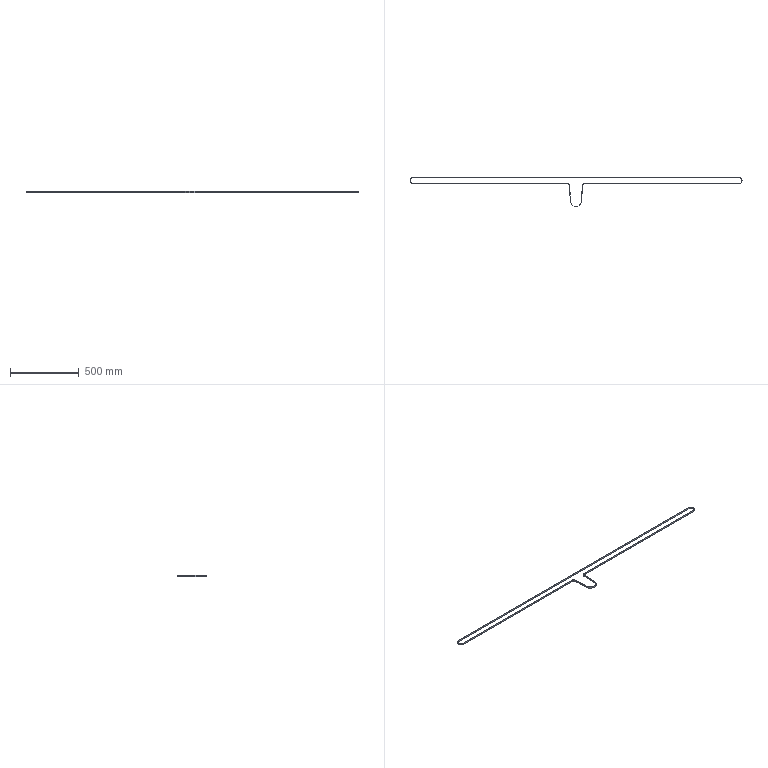Part | NX | features BREP 1 | 1 solid | 24 faces | box 2421 x 214.1 x 12 mm | volume 74422 mm3 | cylinder 12 | plane 12 | commonest cylinder face diameters 45 x3 47.4 x3 25 x2 27.4 x2 80 x1 82.4 x1
STEP:
#1=CARTESIAN_POINT('',(1728.714,8.857,-2.25));
#2=VERTEX_POINT('',#1);
#3=CARTESIAN_POINT('',(1706.214,31.357,-2.25));
#4=VERTEX_POINT('',#3);
#5=CARTESIAN_POINT('',(1706.214,8.857,-2.25));
#6=DIRECTION('',(0.,0.,1.));
#7=DIRECTION('',(-1.,0.,0.));
#8=AXIS2_PLACEMENT_3D('',#5,#6,#7);
#9=CIRCLE('',#8,22.5);
#10=EDGE_CURVE('',#2,#4,#9,.T.);
#11=ORIENTED_EDGE('',*,*,#10,.F.);
#12=CARTESIAN_POINT('',(1728.714,8.857,9.75));
#13=VERTEX_POINT('',#12);
#14=CARTESIAN_POINT('',(1728.714,8.857,-2.25));
#15=DIRECTION('',(0.,0.,1.));
#16=VECTOR('',#15,1000.);
#17=LINE('',#14,#16);
#18=EDGE_CURVE('',#2,#13,#17,.T.);
#19=ORIENTED_EDGE('',*,*,#18,.T.);
#20=CARTESIAN_POINT('',(1706.214,31.357,9.75));
#21=VERTEX_POINT('',#20);
#22=CARTESIAN_POINT('',(1706.214,8.857,9.75));
#23=DIRECTION('',(0.,0.,1.));
#24=DIRECTION('',(-1.,0.,0.));
#25=AXIS2_PLACEMENT_3D('',#22,#23,#24);
#26=CIRCLE('',#25,22.5);
#27=EDGE_CURVE('',#13,#21,#26,.T.);
#28=ORIENTED_EDGE('',*,*,#27,.T.);
#29=CARTESIAN_POINT('',(1706.214,31.357,-2.25));
#30=DIRECTION('',(0.,0.,1.));
#31=VECTOR('',#30,1000.);
#32=LINE('',#29,#31);
#33=EDGE_CURVE('',#4,#21,#32,.T.);
#34=ORIENTED_EDGE('',*,*,#33,.F.);
#35=EDGE_LOOP('',(#11,#19,#28,#34));
#36=FACE_BOUND('',#35,.T.);
#37=CARTESIAN_POINT('',(1706.214,8.857,-2.25));
#38=DIRECTION('',(0.,0.,1.));
#39=DIRECTION('',(1.,0.,0.));
#40=AXIS2_PLACEMENT_3D('',#37,#38,#39);
#41=CYLINDRICAL_SURFACE('',#40,22.5);
#42=ADVANCED_FACE('',(#36),#41,.F.);
#43=CARTESIAN_POINT('',(1706.214,-14.843,-2.25));
#44=VERTEX_POINT('',#43);
#45=CARTESIAN_POINT('',(1729.914,8.857,-2.25));
#46=VERTEX_POINT('',#45);
#47=CARTESIAN_POINT('',(1706.214,8.857,-2.25));
#48=DIRECTION('',(0.,0.,1.));
#49=DIRECTION('',(1.,0.,0.));
#50=AXIS2_PLACEMENT_3D('',#47,#48,#49);
#51=CIRCLE('',#50,23.7);
#52=EDGE_CURVE('',#44,#46,#51,.T.);
#53=ORIENTED_EDGE('',*,*,#52,.T.);
#54=CARTESIAN_POINT('',(1729.914,8.857,9.75));
#55=VERTEX_POINT('',#54);
#56=CARTESIAN_POINT('',(1729.914,8.857,-2.25));
#57=DIRECTION('',(0.,0.,1.));
#58=VECTOR('',#57,1000.);
#59=LINE('',#56,#58);
#60=EDGE_CURVE('',#46,#55,#59,.T.);
#61=ORIENTED_EDGE('',*,*,#60,.T.);
#62=CARTESIAN_POINT('',(1706.214,-14.843,9.75));
#63=VERTEX_POINT('',#62);
#64=CARTESIAN_POINT('',(1706.214,8.857,9.75));
#65=DIRECTION('',(0.,0.,1.));
#66=DIRECTION('',(1.,0.,0.));
#67=AXIS2_PLACEMENT_3D('',#64,#65,#66);
#68=CIRCLE('',#67,23.7);
#69=EDGE_CURVE('',#63,#55,#68,.T.);
#70=ORIENTED_EDGE('',*,*,#69,.F.);
#71=CARTESIAN_POINT('',(1706.214,-14.843,-2.25));
#72=DIRECTION('',(0.,0.,1.));
#73=VECTOR('',#72,1000.);
#74=LINE('',#71,#73);
#75=EDGE_CURVE('',#44,#63,#74,.T.);
#76=ORIENTED_EDGE('',*,*,#75,.F.);
#77=EDGE_LOOP('',(#53,#61,#70,#76));
#78=FACE_BOUND('',#77,.T.);
#79=CARTESIAN_POINT('',(1706.214,8.857,-2.25));
#80=DIRECTION('',(0.,0.,1.));
#81=DIRECTION('',(1.,0.,0.));
#82=AXIS2_PLACEMENT_3D('',#79,#80,#81);
#83=CYLINDRICAL_SURFACE('',#82,23.7);
#84=ADVANCED_FACE('',(#78),#83,.T.);
#85=ORIENTED_EDGE('',*,*,#60,.F.);
#86=CARTESIAN_POINT('',(1706.214,32.557,-2.25));
#87=VERTEX_POINT('',#86);
#88=CARTESIAN_POINT('',(1706.214,8.857,-2.25));
#89=DIRECTION('',(0.,0.,1.));
#90=DIRECTION('',(1.,0.,0.));
#91=AXIS2_PLACEMENT_3D('',#88,#89,#90);
#92=CIRCLE('',#91,23.7);
#93=EDGE_CURVE('',#46,#87,#92,.T.);
#94=ORIENTED_EDGE('',*,*,#93,.T.);
#95=CARTESIAN_POINT('',(1706.214,32.557,9.75));
#96=VERTEX_POINT('',#95);
#97=CARTESIAN_POINT('',(1706.214,32.557,-2.25));
#98=DIRECTION('',(0.,0.,1.));
#99=VECTOR('',#98,1000.);
#100=LINE('',#97,#99);
#101=EDGE_CURVE('',#87,#96,#100,.T.);
#102=ORIENTED_EDGE('',*,*,#101,.T.);
#103=CARTESIAN_POINT('',(1706.214,8.857,9.75));
#104=DIRECTION('',(0.,0.,1.));
#105=DIRECTION('',(1.,0.,0.));
#106=AXIS2_PLACEMENT_3D('',#103,#104,#105);
#107=CIRCLE('',#106,23.7);
#108=EDGE_CURVE('',#55,#96,#107,.T.);
#109=ORIENTED_EDGE('',*,*,#108,.F.);
#110=EDGE_LOOP('',(#85,#94,#102,#109));
#111=FACE_BOUND('',#110,.T.);
#112=CARTESIAN_POINT('',(1706.214,8.857,-2.25));
#113=DIRECTION('',(0.,0.,1.));
#114=DIRECTION('',(1.,0.,0.));
#115=AXIS2_PLACEMENT_3D('',#112,#113,#114);
#116=CYLINDRICAL_SURFACE('',#115,23.7);
#117=ADVANCED_FACE('',(#111),#116,.T.);
#118=CARTESIAN_POINT('',(579.214,-14.843,9.75));
#119=VERTEX_POINT('',#118);
#120=CARTESIAN_POINT('',(579.214,-14.843,9.75));
#121=DIRECTION('',(1.,0.,0.));
#122=VECTOR('',#121,1000.);
#123=LINE('',#120,#122);
#124=EDGE_CURVE('',#119,#63,#123,.T.);
#125=ORIENTED_EDGE('',*,*,#124,.F.);
#126=CARTESIAN_POINT('',(579.214,-14.843,-2.25));
#127=VERTEX_POINT('',#126);
#128=CARTESIAN_POINT('',(579.214,-14.843,-2.25));
#129=DIRECTION('',(0.,0.,1.));
#130=VECTOR('',#129,1000.);
#131=LINE('',#128,#130);
#132=EDGE_CURVE('',#127,#119,#131,.T.);
#133=ORIENTED_EDGE('',*,*,#132,.F.);
#134=CARTESIAN_POINT('',(579.214,-14.843,-2.25));
#135=DIRECTION('',(1.,0.,0.));
#136=VECTOR('',#135,1000.);
#137=LINE('',#134,#136);
#138=EDGE_CURVE('',#127,#44,#137,.T.);
#139=ORIENTED_EDGE('',*,*,#138,.T.);
#140=ORIENTED_EDGE('',*,*,#75,.T.);
#141=EDGE_LOOP('',(#125,#133,#139,#140));
#142=FACE_BOUND('',#141,.T.);
#143=CARTESIAN_POINT('',(579.214,-14.843,-2.25));
#144=DIRECTION('',(0.,-1.,0.));
#145=DIRECTION('',(0.,0.,-1.));
#146=AXIS2_PLACEMENT_3D('',#143,#144,#145);
#147=PLANE('',#146);
#148=ADVANCED_FACE('',(#142),#147,.T.);
#149=CARTESIAN_POINT('',(566.733,-26.656,9.75));
#150=VERTEX_POINT('',#149);
#151=CARTESIAN_POINT('',(579.214,-27.343,9.75));
#152=DIRECTION('',(0.,0.,-1.));
#153=DIRECTION('',(-1.,0.,0.));
#154=AXIS2_PLACEMENT_3D('',#151,#152,#153);
#155=CIRCLE('',#154,12.5);
#156=EDGE_CURVE('',#150,#119,#155,.T.);
#157=ORIENTED_EDGE('',*,*,#156,.F.);
#158=CARTESIAN_POINT('',(566.733,-26.656,-2.25));
#159=VERTEX_POINT('',#158);
#160=CARTESIAN_POINT('',(566.733,-26.656,-2.25));
#161=DIRECTION('',(0.,0.,1.));
#162=VECTOR('',#161,1000.);
#163=LINE('',#160,#162);
#164=EDGE_CURVE('',#159,#150,#163,.T.);
#165=ORIENTED_EDGE('',*,*,#164,.F.);
#166=CARTESIAN_POINT('',(579.214,-27.343,-2.25));
#167=DIRECTION('',(0.,0.,-1.));
#168=DIRECTION('',(-1.,0.,0.));
#169=AXIS2_PLACEMENT_3D('',#166,#167,#168);
#170=CIRCLE('',#169,12.5);
#171=EDGE_CURVE('',#159,#127,#170,.T.);
#172=ORIENTED_EDGE('',*,*,#171,.T.);
#173=ORIENTED_EDGE('',*,*,#132,.T.);
#174=EDGE_LOOP('',(#157,#165,#172,#173));
#175=FACE_BOUND('',#174,.T.);
#176=CARTESIAN_POINT('',(579.214,-27.343,-2.25));
#177=DIRECTION('',(0.,0.,1.));
#178=DIRECTION('',(1.,0.,0.));
#179=AXIS2_PLACEMENT_3D('',#176,#177,#178);
#180=CYLINDRICAL_SURFACE('',#179,12.5);
#181=ADVANCED_FACE('',(#175),#180,.F.);
#182=CARTESIAN_POINT('',(560.352,-142.607,9.75));
#183=VERTEX_POINT('',#182);
#184=CARTESIAN_POINT('',(560.352,-142.607,9.75));
#185=DIRECTION('',(0.05495,0.9985,0.));
#186=VECTOR('',#185,1000.);
#187=LINE('',#184,#186);
#188=EDGE_CURVE('',#183,#150,#187,.T.);
#189=ORIENTED_EDGE('',*,*,#188,.F.);
#190=CARTESIAN_POINT('',(560.352,-142.607,-2.25));
#191=VERTEX_POINT('',#190);
#192=CARTESIAN_POINT('',(560.352,-142.607,-2.25));
#193=DIRECTION('',(0.,0.,1.));
#194=VECTOR('',#193,1000.);
#195=LINE('',#192,#194);
#196=EDGE_CURVE('',#191,#183,#195,.T.);
#197=ORIENTED_EDGE('',*,*,#196,.F.);
#198=CARTESIAN_POINT('',(560.352,-142.607,-2.25));
#199=DIRECTION('',(0.05495,0.9985,0.));
#200=VECTOR('',#199,1000.);
#201=LINE('',#198,#200);
#202=EDGE_CURVE('',#191,#159,#201,.T.);
#203=ORIENTED_EDGE('',*,*,#202,.T.);
#204=ORIENTED_EDGE('',*,*,#164,.T.);
#205=EDGE_LOOP('',(#189,#197,#203,#204));
#206=FACE_BOUND('',#205,.T.);
#207=CARTESIAN_POINT('',(560.352,-142.607,-2.25));
#208=DIRECTION('',(0.9985,-0.05495,0.));
#209=DIRECTION('',(0.,0.,-1.));
#210=AXIS2_PLACEMENT_3D('',#207,#208,#209);
#211=PLANE('',#210);
#212=ADVANCED_FACE('',(#206),#211,.T.);
#213=CARTESIAN_POINT('',(478.077,-142.607,9.75));
#214=VERTEX_POINT('',#213);
#215=CARTESIAN_POINT('',(519.214,-140.343,9.75));
#216=DIRECTION('',(0.,0.,1.));
#217=DIRECTION('',(1.,0.,0.));
#218=AXIS2_PLACEMENT_3D('',#215,#216,#217);
#219=CIRCLE('',#218,41.2);
#220=EDGE_CURVE('',#214,#183,#219,.T.);
#221=ORIENTED_EDGE('',*,*,#220,.F.);
#222=CARTESIAN_POINT('',(478.077,-142.607,-2.25));
#223=VERTEX_POINT('',#222);
#224=CARTESIAN_POINT('',(478.077,-142.607,-2.25));
#225=DIRECTION('',(0.,0.,1.));
#226=VECTOR('',#225,1000.);
#227=LINE('',#224,#226);
#228=EDGE_CURVE('',#223,#214,#227,.T.);
#229=ORIENTED_EDGE('',*,*,#228,.F.);
#230=CARTESIAN_POINT('',(519.214,-140.343,-2.25));
#231=DIRECTION('',(0.,0.,1.));
#232=DIRECTION('',(1.,0.,0.));
#233=AXIS2_PLACEMENT_3D('',#230,#231,#232);
#234=CIRCLE('',#233,41.2);
#235=EDGE_CURVE('',#223,#191,#234,.T.);
#236=ORIENTED_EDGE('',*,*,#235,.T.);
#237=ORIENTED_EDGE('',*,*,#196,.T.);
#238=EDGE_LOOP('',(#221,#229,#236,#237));
#239=FACE_BOUND('',#238,.T.);
#240=CARTESIAN_POINT('',(519.214,-140.343,-2.25));
#241=DIRECTION('',(0.,0.,1.));
#242=DIRECTION('',(1.,0.,0.));
#243=AXIS2_PLACEMENT_3D('',#240,#241,#242);
#244=CYLINDRICAL_SURFACE('',#243,41.2);
#245=ADVANCED_FACE('',(#239),#244,.T.);
#246=CARTESIAN_POINT('',(471.695,-26.656,9.75));
#247=VERTEX_POINT('',#246);
#248=CARTESIAN_POINT('',(471.695,-26.656,9.75));
#249=DIRECTION('',(0.05495,-0.9985,0.));
#250=VECTOR('',#249,1000.);
#251=LINE('',#248,#250);
#252=EDGE_CURVE('',#247,#214,#251,.T.);
#253=ORIENTED_EDGE('',*,*,#252,.F.);
#254=CARTESIAN_POINT('',(471.695,-26.656,-2.25));
#255=VERTEX_POINT('',#254);
#256=CARTESIAN_POINT('',(471.695,-26.656,-2.25));
#257=DIRECTION('',(0.,0.,1.));
#258=VECTOR('',#257,1000.);
#259=LINE('',#256,#258);
#260=EDGE_CURVE('',#255,#247,#259,.T.);
#261=ORIENTED_EDGE('',*,*,#260,.F.);
#262=CARTESIAN_POINT('',(471.695,-26.656,-2.25));
#263=DIRECTION('',(0.05495,-0.9985,0.));
#264=VECTOR('',#263,1000.);
#265=LINE('',#262,#264);
#266=EDGE_CURVE('',#255,#223,#265,.T.);
#267=ORIENTED_EDGE('',*,*,#266,.T.);
#268=ORIENTED_EDGE('',*,*,#228,.T.);
#269=EDGE_LOOP('',(#253,#261,#267,#268));
#270=FACE_BOUND('',#269,.T.);
#271=CARTESIAN_POINT('',(471.695,-26.656,-2.25));
#272=DIRECTION('',(-0.9985,-0.05495,0.));
#273=DIRECTION('',(-0.05495,0.9985,0.));
#274=AXIS2_PLACEMENT_3D('',#271,#272,#273);
#275=PLANE('',#274);
#276=ADVANCED_FACE('',(#270),#275,.T.);
#277=CARTESIAN_POINT('',(459.214,-14.843,9.75));
#278=VERTEX_POINT('',#277);
#279=CARTESIAN_POINT('',(459.214,-27.343,9.75));
#280=DIRECTION('',(0.,0.,-1.));
#281=DIRECTION('',(-1.,0.,0.));
#282=AXIS2_PLACEMENT_3D('',#279,#280,#281);
#283=CIRCLE('',#282,12.5);
#284=EDGE_CURVE('',#278,#247,#283,.T.);
#285=ORIENTED_EDGE('',*,*,#284,.F.);
#286=CARTESIAN_POINT('',(459.214,-14.843,-2.25));
#287=VERTEX_POINT('',#286);
#288=CARTESIAN_POINT('',(459.214,-14.843,-2.25));
#289=DIRECTION('',(0.,0.,1.));
#290=VECTOR('',#289,1000.);
#291=LINE('',#288,#290);
#292=EDGE_CURVE('',#287,#278,#291,.T.);
#293=ORIENTED_EDGE('',*,*,#292,.F.);
#294=CARTESIAN_POINT('',(459.214,-27.343,-2.25));
#295=DIRECTION('',(0.,0.,-1.));
#296=DIRECTION('',(-1.,0.,0.));
#297=AXIS2_PLACEMENT_3D('',#294,#295,#296);
#298=CIRCLE('',#297,12.5);
#299=EDGE_CURVE('',#287,#255,#298,.T.);
#300=ORIENTED_EDGE('',*,*,#299,.T.);
#301=ORIENTED_EDGE('',*,*,#260,.T.);
#302=EDGE_LOOP('',(#285,#293,#300,#301));
#303=FACE_BOUND('',#302,.T.);
#304=CARTESIAN_POINT('',(459.214,-27.343,-2.25));
#305=DIRECTION('',(0.,0.,1.));
#306=DIRECTION('',(1.,0.,0.));
#307=AXIS2_PLACEMENT_3D('',#304,#305,#306);
#308=CYLINDRICAL_SURFACE('',#307,12.5);
#309=ADVANCED_FACE('',(#303),#308,.F.);
#310=CARTESIAN_POINT('',(-667.786,-14.843,9.75));
#311=VERTEX_POINT('',#310);
#312=CARTESIAN_POINT('',(-667.786,-14.843,9.75));
#313=DIRECTION('',(1.,0.,0.));
#314=VECTOR('',#313,1000.);
#315=LINE('',#312,#314);
#316=EDGE_CURVE('',#311,#278,#315,.T.);
#317=ORIENTED_EDGE('',*,*,#316,.F.);
#318=CARTESIAN_POINT('',(-667.786,-14.843,-2.25));
#319=VERTEX_POINT('',#318);
#320=CARTESIAN_POINT('',(-667.786,-14.843,-2.25));
#321=DIRECTION('',(0.,0.,1.));
#322=VECTOR('',#321,1000.);
#323=LINE('',#320,#322);
#324=EDGE_CURVE('',#319,#311,#323,.T.);
#325=ORIENTED_EDGE('',*,*,#324,.F.);
#326=CARTESIAN_POINT('',(-667.786,-14.843,-2.25));
#327=DIRECTION('',(1.,0.,0.));
#328=VECTOR('',#327,1000.);
#329=LINE('',#326,#328);
#330=EDGE_CURVE('',#319,#287,#329,.T.);
#331=ORIENTED_EDGE('',*,*,#330,.T.);
#332=ORIENTED_EDGE('',*,*,#292,.T.);
#333=EDGE_LOOP('',(#317,#325,#331,#332));
#334=FACE_BOUND('',#333,.T.);
#335=CARTESIAN_POINT('',(-667.786,-14.843,-2.25));
#336=DIRECTION('',(0.,-1.,0.));
#337=DIRECTION('',(-1.,0.,0.));
#338=AXIS2_PLACEMENT_3D('',#335,#336,#337);
#339=PLANE('',#338);
#340=ADVANCED_FACE('',(#334),#339,.T.);
#341=CARTESIAN_POINT('',(-667.786,32.557,9.75));
#342=VERTEX_POINT('',#341);
#343=CARTESIAN_POINT('',(-667.786,8.857,9.75));
#344=DIRECTION('',(0.,0.,1.));
#345=DIRECTION('',(1.,0.,0.));
#346=AXIS2_PLACEMENT_3D('',#343,#344,#345);
#347=CIRCLE('',#346,23.7);
#348=EDGE_CURVE('',#342,#311,#347,.T.);
#349=ORIENTED_EDGE('',*,*,#348,.F.);
#350=CARTESIAN_POINT('',(-667.786,32.557,-2.25));
#351=VERTEX_POINT('',#350);
#352=CARTESIAN_POINT('',(-667.786,32.557,-2.25));
#353=DIRECTION('',(0.,0.,1.));
#354=VECTOR('',#353,1000.);
#355=LINE('',#352,#354);
#356=EDGE_CURVE('',#351,#342,#355,.T.);
#357=ORIENTED_EDGE('',*,*,#356,.F.);
#358=CARTESIAN_POINT('',(-667.786,8.857,-2.25));
#359=DIRECTION('',(0.,0.,1.));
#360=DIRECTION('',(1.,0.,0.));
#361=AXIS2_PLACEMENT_3D('',#358,#359,#360);
#362=CIRCLE('',#361,23.7);
#363=EDGE_CURVE('',#351,#319,#362,.T.);
#364=ORIENTED_EDGE('',*,*,#363,.T.);
#365=ORIENTED_EDGE('',*,*,#324,.T.);
#366=EDGE_LOOP('',(#349,#357,#364,#365));
#367=FACE_BOUND('',#366,.T.);
#368=CARTESIAN_POINT('',(-667.786,8.857,-2.25));
#369=DIRECTION('',(0.,0.,1.));
#370=DIRECTION('',(1.,0.,0.));
#371=AXIS2_PLACEMENT_3D('',#368,#369,#370);
#372=CYLINDRICAL_SURFACE('',#371,23.7);
#373=ADVANCED_FACE('',(#367),#372,.T.);
#374=CARTESIAN_POINT('',(1706.214,32.557,9.75));
#375=DIRECTION('',(-1.,0.,0.));
#376=VECTOR('',#375,1000.);
#377=LINE('',#374,#376);
#378=EDGE_CURVE('',#96,#342,#377,.T.);
#379=ORIENTED_EDGE('',*,*,#378,.F.);
#380=ORIENTED_EDGE('',*,*,#101,.F.);
#381=CARTESIAN_POINT('',(1706.214,32.557,-2.25));
#382=DIRECTION('',(-1.,0.,0.));
#383=VECTOR('',#382,1000.);
#384=LINE('',#381,#383);
#385=EDGE_CURVE('',#87,#351,#384,.T.);
#386=ORIENTED_EDGE('',*,*,#385,.T.);
#387=ORIENTED_EDGE('',*,*,#356,.T.);
#388=EDGE_LOOP('',(#379,#380,#386,#387));
#389=FACE_BOUND('',#388,.T.);
#390=CARTESIAN_POINT('',(1706.214,32.557,-2.25));
#391=DIRECTION('',(0.,1.,0.));
#392=DIRECTION('',(1.,0.,0.));
#393=AXIS2_PLACEMENT_3D('',#390,#391,#392);
#394=PLANE('',#393);
#395=ADVANCED_FACE('',(#389),#394,.T.);
#396=ORIENTED_EDGE('',*,*,#52,.F.);
#397=ORIENTED_EDGE('',*,*,#138,.F.);
#398=ORIENTED_EDGE('',*,*,#171,.F.);
#399=ORIENTED_EDGE('',*,*,#202,.F.);
#400=ORIENTED_EDGE('',*,*,#235,.F.);
#401=ORIENTED_EDGE('',*,*,#266,.F.);
#402=ORIENTED_EDGE('',*,*,#299,.F.);
#403=ORIENTED_EDGE('',*,*,#330,.F.);
#404=ORIENTED_EDGE('',*,*,#363,.F.);
#405=ORIENTED_EDGE('',*,*,#385,.F.);
#406=ORIENTED_EDGE('',*,*,#93,.F.);
#407=EDGE_LOOP('',(#396,#397,#398,#399,#400,#401,#402,#403,#404,#405,#406));
#408=FACE_BOUND('',#407,.T.);
#409=CARTESIAN_POINT('',(472.894,-26.59,-2.25));
#410=VERTEX_POINT('',#409);
#411=CARTESIAN_POINT('',(479.275,-142.541,-2.25));
#412=VERTEX_POINT('',#411);
#413=CARTESIAN_POINT('',(479.275,-142.541,-2.25));
#414=DIRECTION('',(0.05495,-0.9985,0.));
#415=VECTOR('',#414,1000.);
#416=LINE('',#413,#415);
#417=EDGE_CURVE('',#410,#412,#416,.T.);
#418=ORIENTED_EDGE('',*,*,#417,.T.);
#419=CARTESIAN_POINT('',(559.154,-142.541,-2.25));
#420=VERTEX_POINT('',#419);
#421=CARTESIAN_POINT('',(519.214,-140.343,-2.25));
#422=DIRECTION('',(0.,0.,1.));
#423=DIRECTION('',(-1.,0.,0.));
#424=AXIS2_PLACEMENT_3D('',#421,#422,#423);
#425=CIRCLE('',#424,40.);
#426=EDGE_CURVE('',#412,#420,#425,.T.);
#427=ORIENTED_EDGE('',*,*,#426,.T.);
#428=CARTESIAN_POINT('',(565.535,-26.59,-2.25));
#429=VERTEX_POINT('',#428);
#430=CARTESIAN_POINT('',(565.535,-26.59,-2.25));
#431=DIRECTION('',(0.05495,0.9985,0.));
#432=VECTOR('',#431,1000.);
#433=LINE('',#430,#432);
#434=EDGE_CURVE('',#420,#429,#433,.T.);
#435=ORIENTED_EDGE('',*,*,#434,.T.);
#436=CARTESIAN_POINT('',(579.214,-13.643,-2.25));
#437=VERTEX_POINT('',#436);
#438=CARTESIAN_POINT('',(579.214,-27.343,-2.25));
#439=DIRECTION('',(0.,0.,-1.));
#440=DIRECTION('',(1.,0.,0.));
#441=AXIS2_PLACEMENT_3D('',#438,#439,#440);
#442=CIRCLE('',#441,13.7);
#443=EDGE_CURVE('',#429,#437,#442,.T.);
#444=ORIENTED_EDGE('',*,*,#443,.T.);
#445=CARTESIAN_POINT('',(1706.214,-13.643,-2.25));
#446=VERTEX_POINT('',#445);
#447=CARTESIAN_POINT('',(1706.214,-13.643,-2.25));
#448=DIRECTION('',(1.,0.,0.));
#449=VECTOR('',#448,1000.);
#450=LINE('',#447,#449);
#451=EDGE_CURVE('',#437,#446,#450,.T.);
#452=ORIENTED_EDGE('',*,*,#451,.T.);
#453=CARTESIAN_POINT('',(1706.214,8.857,-2.25));
#454=DIRECTION('',(0.,0.,1.));
#455=DIRECTION('',(-1.,0.,0.));
#456=AXIS2_PLACEMENT_3D('',#453,#454,#455);
#457=CIRCLE('',#456,22.5);
#458=EDGE_CURVE('',#446,#2,#457,.T.);
#459=ORIENTED_EDGE('',*,*,#458,.T.);
#460=ORIENTED_EDGE('',*,*,#10,.T.);
#461=CARTESIAN_POINT('',(-667.786,31.357,-2.25));
#462=VERTEX_POINT('',#461);
#463=CARTESIAN_POINT('',(-667.786,31.357,-2.25));
#464=DIRECTION('',(-1.,0.,0.));
#465=VECTOR('',#464,1000.);
#466=LINE('',#463,#465);
#467=EDGE_CURVE('',#4,#462,#466,.T.);
#468=ORIENTED_EDGE('',*,*,#467,.T.);
#469=CARTESIAN_POINT('',(-667.786,-13.643,-2.25));
#470=VERTEX_POINT('',#469);
#471=CARTESIAN_POINT('',(-667.786,8.857,-2.25));
#472=DIRECTION('',(0.,0.,1.));
#473=DIRECTION('',(-1.,0.,0.));
#474=AXIS2_PLACEMENT_3D('',#471,#472,#473);
#475=CIRCLE('',#474,22.5);
#476=EDGE_CURVE('',#462,#470,#475,.T.);
#477=ORIENTED_EDGE('',*,*,#476,.T.);
#478=CARTESIAN_POINT('',(459.214,-13.643,-2.25));
#479=VERTEX_POINT('',#478);
#480=CARTESIAN_POINT('',(459.214,-13.643,-2.25));
#481=DIRECTION('',(1.,0.,0.));
#482=VECTOR('',#481,1000.);
#483=LINE('',#480,#482);
#484=EDGE_CURVE('',#470,#479,#483,.T.);
#485=ORIENTED_EDGE('',*,*,#484,.T.);
#486=CARTESIAN_POINT('',(459.214,-27.343,-2.25));
#487=DIRECTION('',(0.,0.,-1.));
#488=DIRECTION('',(1.,0.,0.));
#489=AXIS2_PLACEMENT_3D('',#486,#487,#488);
#490=CIRCLE('',#489,13.7);
#491=EDGE_CURVE('',#479,#410,#490,.T.);
#492=ORIENTED_EDGE('',*,*,#491,.T.);
#493=EDGE_LOOP('',(#418,#427,#435,#444,#452,#459,#460,#468,#477,#485,#492));
#494=FACE_BOUND('',#493,.T.);
#495=CARTESIAN_POINT('',(1706.214,8.857,-2.25));
#496=DIRECTION('',(0.,0.,1.));
#497=DIRECTION('',(1.,0.,0.));
#498=AXIS2_PLACEMENT_3D('',#495,#496,#497);
#499=PLANE('',#498);
#500=ADVANCED_FACE('',(#408,#494),#499,.F.);
#501=ORIENTED_EDGE('',*,*,#69,.T.);
#502=ORIENTED_EDGE('',*,*,#108,.T.);
#503=ORIENTED_EDGE('',*,*,#378,.T.);
#504=ORIENTED_EDGE('',*,*,#348,.T.);
#505=ORIENTED_EDGE('',*,*,#316,.T.);
#506=ORIENTED_EDGE('',*,*,#284,.T.);
#507=ORIENTED_EDGE('',*,*,#252,.T.);
#508=ORIENTED_EDGE('',*,*,#220,.T.);
#509=ORIENTED_EDGE('',*,*,#188,.T.);
#510=ORIENTED_EDGE('',*,*,#156,.T.);
#511=ORIENTED_EDGE('',*,*,#124,.T.);
#512=EDGE_LOOP('',(#501,#502,#503,#504,#505,#506,#507,#508,#509,#510,#511));
#513=FACE_BOUND('',#512,.T.);
#514=CARTESIAN_POINT('',(479.275,-142.541,9.75));
#515=VERTEX_POINT('',#514);
#516=CARTESIAN_POINT('',(559.154,-142.541,9.75));
#517=VERTEX_POINT('',#516);
#518=CARTESIAN_POINT('',(519.214,-140.343,9.75));
#519=DIRECTION('',(0.,0.,1.));
#520=DIRECTION('',(-1.,0.,0.));
#521=AXIS2_PLACEMENT_3D('',#518,#519,#520);
#522=CIRCLE('',#521,40.);
#523=EDGE_CURVE('',#515,#517,#522,.T.);
#524=ORIENTED_EDGE('',*,*,#523,.F.);
#525=CARTESIAN_POINT('',(472.894,-26.59,9.75));
#526=VERTEX_POINT('',#525);
#527=CARTESIAN_POINT('',(479.275,-142.541,9.75));
#528=DIRECTION('',(0.05495,-0.9985,0.));
#529=VECTOR('',#528,1000.);
#530=LINE('',#527,#529);
#531=EDGE_CURVE('',#526,#515,#530,.T.);
#532=ORIENTED_EDGE('',*,*,#531,.F.);
#533=CARTESIAN_POINT('',(459.214,-13.643,9.75));
#534=VERTEX_POINT('',#533);
#535=CARTESIAN_POINT('',(459.214,-27.343,9.75));
#536=DIRECTION('',(0.,0.,-1.));
#537=DIRECTION('',(1.,0.,0.));
#538=AXIS2_PLACEMENT_3D('',#535,#536,#537);
#539=CIRCLE('',#538,13.7);
#540=EDGE_CURVE('',#534,#526,#539,.T.);
#541=ORIENTED_EDGE('',*,*,#540,.F.);
#542=CARTESIAN_POINT('',(-667.786,-13.643,9.75));
#543=VERTEX_POINT('',#542);
#544=CARTESIAN_POINT('',(459.214,-13.643,9.75));
#545=DIRECTION('',(1.,0.,0.));
#546=VECTOR('',#545,1000.);
#547=LINE('',#544,#546);
#548=EDGE_CURVE('',#543,#534,#547,.T.);
#549=ORIENTED_EDGE('',*,*,#548,.F.);
#550=CARTESIAN_POINT('',(-667.786,31.357,9.75));
#551=VERTEX_POINT('',#550);
#552=CARTESIAN_POINT('',(-667.786,8.857,9.75));
#553=DIRECTION('',(0.,0.,1.));
#554=DIRECTION('',(-1.,0.,0.));
#555=AXIS2_PLACEMENT_3D('',#552,#553,#554);
#556=CIRCLE('',#555,22.5);
#557=EDGE_CURVE('',#551,#543,#556,.T.);
#558=ORIENTED_EDGE('',*,*,#557,.F.);
#559=CARTESIAN_POINT('',(-667.786,31.357,9.75));
#560=DIRECTION('',(-1.,0.,0.));
#561=VECTOR('',#560,1000.);
#562=LINE('',#559,#561);
#563=EDGE_CURVE('',#21,#551,#562,.T.);
#564=ORIENTED_EDGE('',*,*,#563,.F.);
#565=ORIENTED_EDGE('',*,*,#27,.F.);
#566=CARTESIAN_POINT('',(1706.214,-13.643,9.75));
#567=VERTEX_POINT('',#566);
#568=CARTESIAN_POINT('',(1706.214,8.857,9.75));
#569=DIRECTION('',(0.,0.,1.));
#570=DIRECTION('',(-1.,0.,0.));
#571=AXIS2_PLACEMENT_3D('',#568,#569,#570);
#572=CIRCLE('',#571,22.5);
#573=EDGE_CURVE('',#567,#13,#572,.T.);
#574=ORIENTED_EDGE('',*,*,#573,.F.);
#575=CARTESIAN_POINT('',(579.214,-13.643,9.75));
#576=VERTEX_POINT('',#575);
#577=CARTESIAN_POINT('',(1706.214,-13.643,9.75));
#578=DIRECTION('',(1.,0.,0.));
#579=VECTOR('',#578,1000.);
#580=LINE('',#577,#579);
#581=EDGE_CURVE('',#576,#567,#580,.T.);
#582=ORIENTED_EDGE('',*,*,#581,.F.);
#583=CARTESIAN_POINT('',(565.535,-26.59,9.75));
#584=VERTEX_POINT('',#583);
#585=CARTESIAN_POINT('',(579.214,-27.343,9.75));
#586=DIRECTION('',(0.,0.,-1.));
#587=DIRECTION('',(1.,0.,0.));
#588=AXIS2_PLACEMENT_3D('',#585,#586,#587);
#589=CIRCLE('',#588,13.7);
#590=EDGE_CURVE('',#584,#576,#589,.T.);
#591=ORIENTED_EDGE('',*,*,#590,.F.);
#592=CARTESIAN_POINT('',(565.535,-26.59,9.75));
#593=DIRECTION('',(0.05495,0.9985,0.));
#594=VECTOR('',#593,1000.);
#595=LINE('',#592,#594);
#596=EDGE_CURVE('',#517,#584,#595,.T.);
#597=ORIENTED_EDGE('',*,*,#596,.F.);
#598=EDGE_LOOP('',(#524,#532,#541,#549,#558,#564,#565,#574,#582,#591,#597));
#599=FACE_BOUND('',#598,.T.);
#600=CARTESIAN_POINT('',(1706.214,8.857,9.75));
#601=DIRECTION('',(0.,0.,1.));
#602=DIRECTION('',(1.,0.,0.));
#603=AXIS2_PLACEMENT_3D('',#600,#601,#602);
#604=PLANE('',#603);
#605=ADVANCED_FACE('',(#513,#599),#604,.T.);
#606=ORIENTED_EDGE('',*,*,#523,.T.);
#607=CARTESIAN_POINT('',(559.154,-142.541,-2.25));
#608=DIRECTION('',(0.,0.,1.));
#609=VECTOR('',#608,1000.);
#610=LINE('',#607,#609);
#611=EDGE_CURVE('',#420,#517,#610,.T.);
#612=ORIENTED_EDGE('',*,*,#611,.F.);
#613=ORIENTED_EDGE('',*,*,#426,.F.);
#614=CARTESIAN_POINT('',(479.275,-142.541,-2.25));
#615=DIRECTION('',(0.,0.,1.));
#616=VECTOR('',#615,1000.);
#617=LINE('',#614,#616);
#618=EDGE_CURVE('',#412,#515,#617,.T.);
#619=ORIENTED_EDGE('',*,*,#618,.T.);
#620=EDGE_LOOP('',(#606,#612,#613,#619));
#621=FACE_BOUND('',#620,.T.);
#622=CARTESIAN_POINT('',(519.214,-140.343,-2.25));
#623=DIRECTION('',(0.,0.,1.));
#624=DIRECTION('',(1.,0.,0.));
#625=AXIS2_PLACEMENT_3D('',#622,#623,#624);
#626=CYLINDRICAL_SURFACE('',#625,40.);
#627=ADVANCED_FACE('',(#621),#626,.F.);
#628=ORIENTED_EDGE('',*,*,#531,.T.);
#629=ORIENTED_EDGE('',*,*,#618,.F.);
#630=ORIENTED_EDGE('',*,*,#417,.F.);
#631=CARTESIAN_POINT('',(472.894,-26.59,-2.25));
#632=DIRECTION('',(0.,0.,1.));
#633=VECTOR('',#632,1000.);
#634=LINE('',#631,#633);
#635=EDGE_CURVE('',#410,#526,#634,.T.);
#636=ORIENTED_EDGE('',*,*,#635,.T.);
#637=EDGE_LOOP('',(#628,#629,#630,#636));
#638=FACE_BOUND('',#637,.T.);
#639=CARTESIAN_POINT('',(479.275,-142.541,-2.25));
#640=DIRECTION('',(-0.9985,-0.05495,0.));
#641=DIRECTION('',(-0.05495,0.9985,0.));
#642=AXIS2_PLACEMENT_3D('',#639,#640,#641);
#643=PLANE('',#642);
#644=ADVANCED_FACE('',(#638),#643,.F.);
#645=ORIENTED_EDGE('',*,*,#540,.T.);
#646=ORIENTED_EDGE('',*,*,#635,.F.);
#647=ORIENTED_EDGE('',*,*,#491,.F.);
#648=CARTESIAN_POINT('',(459.214,-13.643,-2.25));
#649=DIRECTION('',(0.,0.,1.));
#650=VECTOR('',#649,1000.);
#651=LINE('',#648,#650);
#652=EDGE_CURVE('',#479,#534,#651,.T.);
#653=ORIENTED_EDGE('',*,*,#652,.T.);
#654=EDGE_LOOP('',(#645,#646,#647,#653));
#655=FACE_BOUND('',#654,.T.);
#656=CARTESIAN_POINT('',(459.214,-27.343,-2.25));
#657=DIRECTION('',(0.,0.,1.));
#658=DIRECTION('',(1.,0.,0.));
#659=AXIS2_PLACEMENT_3D('',#656,#657,#658);
#660=CYLINDRICAL_SURFACE('',#659,13.7);
#661=ADVANCED_FACE('',(#655),#660,.T.);
#662=ORIENTED_EDGE('',*,*,#548,.T.);
#663=ORIENTED_EDGE('',*,*,#652,.F.);
#664=ORIENTED_EDGE('',*,*,#484,.F.);
#665=CARTESIAN_POINT('',(-667.786,-13.643,-2.25));
#666=DIRECTION('',(0.,0.,1.));
#667=VECTOR('',#666,1000.);
#668=LINE('',#665,#667);
#669=EDGE_CURVE('',#470,#543,#668,.T.);
#670=ORIENTED_EDGE('',*,*,#669,.T.);
#671=EDGE_LOOP('',(#662,#663,#664,#670));
#672=FACE_BOUND('',#671,.T.);
#673=CARTESIAN_POINT('',(459.214,-13.643,-2.25));
#674=DIRECTION('',(0.,-1.,0.));
#675=DIRECTION('',(0.,0.,-1.));
#676=AXIS2_PLACEMENT_3D('',#673,#674,#675);
#677=PLANE('',#676);
#678=ADVANCED_FACE('',(#672),#677,.F.);
#679=ORIENTED_EDGE('',*,*,#557,.T.);
#680=ORIENTED_EDGE('',*,*,#669,.F.);
#681=ORIENTED_EDGE('',*,*,#476,.F.);
#682=CARTESIAN_POINT('',(-667.786,31.357,-2.25));
#683=DIRECTION('',(0.,0.,1.));
#684=VECTOR('',#683,1000.);
#685=LINE('',#682,#684);
#686=EDGE_CURVE('',#462,#551,#685,.T.);
#687=ORIENTED_EDGE('',*,*,#686,.T.);
#688=EDGE_LOOP('',(#679,#680,#681,#687));
#689=FACE_BOUND('',#688,.T.);
#690=CARTESIAN_POINT('',(-667.786,8.857,-2.25));
#691=DIRECTION('',(0.,0.,1.));
#692=DIRECTION('',(1.,0.,0.));
#693=AXIS2_PLACEMENT_3D('',#690,#691,#692);
#694=CYLINDRICAL_SURFACE('',#693,22.5);
#695=ADVANCED_FACE('',(#689),#694,.F.);
#696=ORIENTED_EDGE('',*,*,#563,.T.);
#697=ORIENTED_EDGE('',*,*,#686,.F.);
#698=ORIENTED_EDGE('',*,*,#467,.F.);
#699=ORIENTED_EDGE('',*,*,#33,.T.);
#700=EDGE_LOOP('',(#696,#697,#698,#699));
#701=FACE_BOUND('',#700,.T.);
#702=CARTESIAN_POINT('',(-667.786,31.357,-2.25));
#703=DIRECTION('',(0.,1.,0.));
#704=DIRECTION('',(1.,0.,0.));
#705=AXIS2_PLACEMENT_3D('',#702,#703,#704);
#706=PLANE('',#705);
#707=ADVANCED_FACE('',(#701),#706,.F.);
#708=ORIENTED_EDGE('',*,*,#18,.F.);
#709=ORIENTED_EDGE('',*,*,#458,.F.);
#710=CARTESIAN_POINT('',(1706.214,-13.643,-2.25));
#711=DIRECTION('',(0.,0.,1.));
#712=VECTOR('',#711,1000.);
#713=LINE('',#710,#712);
#714=EDGE_CURVE('',#446,#567,#713,.T.);
#715=ORIENTED_EDGE('',*,*,#714,.T.);
#716=ORIENTED_EDGE('',*,*,#573,.T.);
#717=EDGE_LOOP('',(#708,#709,#715,#716));
#718=FACE_BOUND('',#717,.T.);
#719=CARTESIAN_POINT('',(1706.214,8.857,-2.25));
#720=DIRECTION('',(0.,0.,1.));
#721=DIRECTION('',(1.,0.,0.));
#722=AXIS2_PLACEMENT_3D('',#719,#720,#721);
#723=CYLINDRICAL_SURFACE('',#722,22.5);
#724=ADVANCED_FACE('',(#718),#723,.F.);
#725=ORIENTED_EDGE('',*,*,#581,.T.);
#726=ORIENTED_EDGE('',*,*,#714,.F.);
#727=ORIENTED_EDGE('',*,*,#451,.F.);
#728=CARTESIAN_POINT('',(579.214,-13.643,-2.25));
#729=DIRECTION('',(0.,0.,1.));
#730=VECTOR('',#729,1000.);
#731=LINE('',#728,#730);
#732=EDGE_CURVE('',#437,#576,#731,.T.);
#733=ORIENTED_EDGE('',*,*,#732,.T.);
#734=EDGE_LOOP('',(#725,#726,#727,#733));
#735=FACE_BOUND('',#734,.T.);
#736=CARTESIAN_POINT('',(1706.214,-13.643,-2.25));
#737=DIRECTION('',(0.,-1.,0.));
#738=DIRECTION('',(0.,0.,-1.));
#739=AXIS2_PLACEMENT_3D('',#736,#737,#738);
#740=PLANE('',#739);
#741=ADVANCED_FACE('',(#735),#740,.F.);
#742=ORIENTED_EDGE('',*,*,#590,.T.);
#743=ORIENTED_EDGE('',*,*,#732,.F.);
#744=ORIENTED_EDGE('',*,*,#443,.F.);
#745=CARTESIAN_POINT('',(565.535,-26.59,-2.25));
#746=DIRECTION('',(0.,0.,1.));
#747=VECTOR('',#746,1000.);
#748=LINE('',#745,#747);
#749=EDGE_CURVE('',#429,#584,#748,.T.);
#750=ORIENTED_EDGE('',*,*,#749,.T.);
#751=EDGE_LOOP('',(#742,#743,#744,#750));
#752=FACE_BOUND('',#751,.T.);
#753=CARTESIAN_POINT('',(579.214,-27.343,-2.25));
#754=DIRECTION('',(0.,0.,1.));
#755=DIRECTION('',(1.,0.,0.));
#756=AXIS2_PLACEMENT_3D('',#753,#754,#755);
#757=CYLINDRICAL_SURFACE('',#756,13.7);
#758=ADVANCED_FACE('',(#752),#757,.T.);
#759=ORIENTED_EDGE('',*,*,#596,.T.);
#760=ORIENTED_EDGE('',*,*,#749,.F.);
#761=ORIENTED_EDGE('',*,*,#434,.F.);
#762=ORIENTED_EDGE('',*,*,#611,.T.);
#763=EDGE_LOOP('',(#759,#760,#761,#762));
#764=FACE_BOUND('',#763,.T.);
#765=CARTESIAN_POINT('',(565.535,-26.59,-2.25));
#766=DIRECTION('',(0.9985,-0.05495,0.));
#767=DIRECTION('',(0.,0.,-1.));
#768=AXIS2_PLACEMENT_3D('',#765,#766,#767);
#769=PLANE('',#768);
#770=ADVANCED_FACE('',(#764),#769,.F.);
#771=CLOSED_SHELL('',(#42,#84,#117,#148,#181,#212,#245,#276,#309,#340,#373,#395,#500,#605,#627,#644,#661,#678,#695,#707,#724,#741,#758,#770));
#772=MANIFOLD_SOLID_BREP('',#771);
#773=(LENGTH_UNIT()NAMED_UNIT(*)SI_UNIT(.MILLI.,.METRE.));
#774=UNCERTAINTY_MEASURE_WITH_UNIT(LENGTH_MEASURE(0.00001),#773,'','');
#775=(NAMED_UNIT(*)PLANE_ANGLE_UNIT()SI_UNIT($,.RADIAN.));
#776=(NAMED_UNIT(*)SI_UNIT($,.STERADIAN.)SOLID_ANGLE_UNIT());
#777=(GEOMETRIC_REPRESENTATION_CONTEXT(3)GLOBAL_UNCERTAINTY_ASSIGNED_CONTEXT((#774))GLOBAL_UNIT_ASSIGNED_CONTEXT((#773,#775,#776))REPRESENTATION_CONTEXT('',''));
#778=ADVANCED_BREP_SHAPE_REPRESENTATION('',(#772),#777);